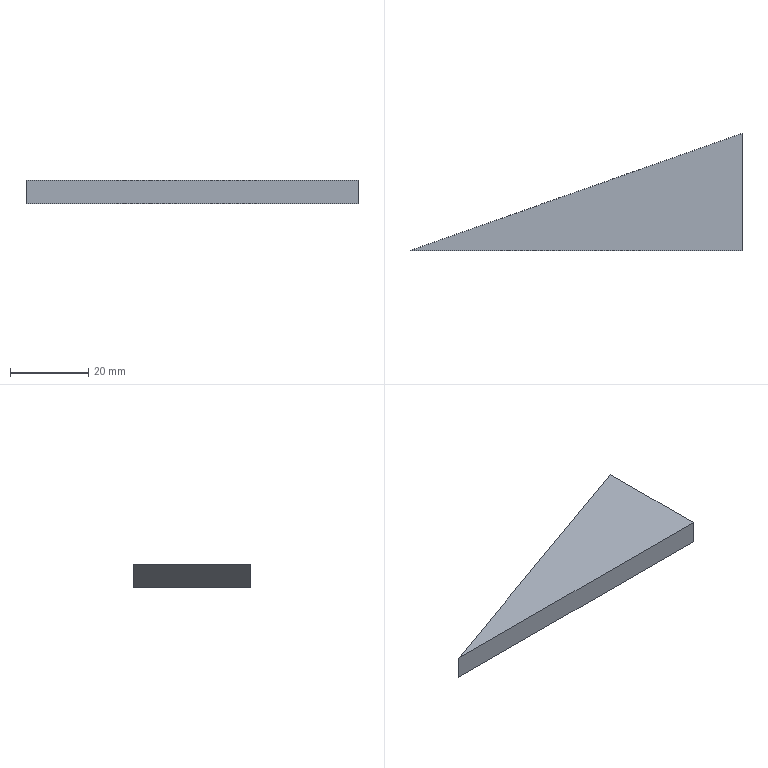Part | STEP file | Guide wheel mechanism revised.sldasm-Part-63 | 1 solid | 5 faces | box 85 x 30 x 6 mm | volume 7650 mm3 | plane 5
STEP:
#1=CARTESIAN_POINT('',(-42.5,7.,-40.5));
#2=VERTEX_POINT('',#1);
#3=CARTESIAN_POINT('',(42.5,37.,-40.5));
#4=VERTEX_POINT('',#3);
#5=CARTESIAN_POINT('',(-42.5,7.,-40.5));
#6=DIRECTION('',(0.943,0.3328,0.));
#7=VECTOR('',#6,1000.);
#8=LINE('',#5,#7);
#9=EDGE_CURVE('',#2,#4,#8,.T.);
#10=ORIENTED_EDGE('',*,*,#9,.F.);
#11=CARTESIAN_POINT('',(-42.5,7.,-34.5));
#12=VERTEX_POINT('',#11);
#13=CARTESIAN_POINT('',(-42.5,7.,-34.5));
#14=DIRECTION('',(0.,0.,-1.));
#15=VECTOR('',#14,1000.);
#16=LINE('',#13,#15);
#17=EDGE_CURVE('',#12,#2,#16,.T.);
#18=ORIENTED_EDGE('',*,*,#17,.F.);
#19=CARTESIAN_POINT('',(42.5,37.,-34.5));
#20=VERTEX_POINT('',#19);
#21=CARTESIAN_POINT('',(-42.5,7.,-34.5));
#22=DIRECTION('',(0.943,0.3328,0.));
#23=VECTOR('',#22,1000.);
#24=LINE('',#21,#23);
#25=EDGE_CURVE('',#12,#20,#24,.T.);
#26=ORIENTED_EDGE('',*,*,#25,.T.);
#27=CARTESIAN_POINT('',(42.5,37.,-34.5));
#28=DIRECTION('',(0.,0.,-1.));
#29=VECTOR('',#28,1000.);
#30=LINE('',#27,#29);
#31=EDGE_CURVE('',#20,#4,#30,.T.);
#32=ORIENTED_EDGE('',*,*,#31,.T.);
#33=EDGE_LOOP('',(#10,#18,#26,#32));
#34=FACE_OUTER_BOUND('',#33,.T.);
#35=CARTESIAN_POINT('',(-42.5,7.,-34.5));
#36=DIRECTION('',(-0.3328,0.943,0.));
#37=DIRECTION('',(-0.943,-0.3328,0.));
#38=AXIS2_PLACEMENT_3D('',#35,#36,#37);
#39=PLANE('',#38);
#40=ADVANCED_FACE('',(#34),#39,.T.);
#41=CARTESIAN_POINT('',(42.5,7.,-40.5));
#42=VERTEX_POINT('',#41);
#43=CARTESIAN_POINT('',(42.5,7.,-40.5));
#44=DIRECTION('',(-1.,0.,0.));
#45=VECTOR('',#44,1000.);
#46=LINE('',#43,#45);
#47=EDGE_CURVE('',#42,#2,#46,.T.);
#48=ORIENTED_EDGE('',*,*,#47,.F.);
#49=CARTESIAN_POINT('',(42.5,7.,-34.5));
#50=VERTEX_POINT('',#49);
#51=CARTESIAN_POINT('',(42.5,7.,-34.5));
#52=DIRECTION('',(0.,0.,-1.));
#53=VECTOR('',#52,1000.);
#54=LINE('',#51,#53);
#55=EDGE_CURVE('',#50,#42,#54,.T.);
#56=ORIENTED_EDGE('',*,*,#55,.F.);
#57=CARTESIAN_POINT('',(42.5,7.,-34.5));
#58=DIRECTION('',(-1.,0.,0.));
#59=VECTOR('',#58,1000.);
#60=LINE('',#57,#59);
#61=EDGE_CURVE('',#50,#12,#60,.T.);
#62=ORIENTED_EDGE('',*,*,#61,.T.);
#63=ORIENTED_EDGE('',*,*,#17,.T.);
#64=EDGE_LOOP('',(#48,#56,#62,#63));
#65=FACE_OUTER_BOUND('',#64,.T.);
#66=CARTESIAN_POINT('',(42.5,7.,-34.5));
#67=DIRECTION('',(0.,-1.,0.));
#68=DIRECTION('',(0.,0.,-1.));
#69=AXIS2_PLACEMENT_3D('',#66,#67,#68);
#70=PLANE('',#69);
#71=ADVANCED_FACE('',(#65),#70,.T.);
#72=CARTESIAN_POINT('',(42.5,37.,-40.5));
#73=DIRECTION('',(0.,-1.,0.));
#74=VECTOR('',#73,1000.);
#75=LINE('',#72,#74);
#76=EDGE_CURVE('',#4,#42,#75,.T.);
#77=ORIENTED_EDGE('',*,*,#76,.F.);
#78=ORIENTED_EDGE('',*,*,#31,.F.);
#79=CARTESIAN_POINT('',(42.5,37.,-34.5));
#80=DIRECTION('',(0.,-1.,0.));
#81=VECTOR('',#80,1000.);
#82=LINE('',#79,#81);
#83=EDGE_CURVE('',#20,#50,#82,.T.);
#84=ORIENTED_EDGE('',*,*,#83,.T.);
#85=ORIENTED_EDGE('',*,*,#55,.T.);
#86=EDGE_LOOP('',(#77,#78,#84,#85));
#87=FACE_OUTER_BOUND('',#86,.T.);
#88=CARTESIAN_POINT('',(42.5,37.,-34.5));
#89=DIRECTION('',(1.,0.,0.));
#90=DIRECTION('',(0.,0.,-1.));
#91=AXIS2_PLACEMENT_3D('',#88,#89,#90);
#92=PLANE('',#91);
#93=ADVANCED_FACE('',(#87),#92,.T.);
#94=ORIENTED_EDGE('',*,*,#25,.F.);
#95=ORIENTED_EDGE('',*,*,#61,.F.);
#96=ORIENTED_EDGE('',*,*,#83,.F.);
#97=EDGE_LOOP('',(#94,#95,#96));
#98=FACE_OUTER_BOUND('',#97,.T.);
#99=CARTESIAN_POINT('',(0.,0.,-34.5));
#100=DIRECTION('',(0.,0.,-1.));
#101=DIRECTION('',(0.,1.,0.));
#102=AXIS2_PLACEMENT_3D('',#99,#100,#101);
#103=PLANE('',#102);
#104=ADVANCED_FACE('',(#98),#103,.F.);
#105=ORIENTED_EDGE('',*,*,#9,.T.);
#106=ORIENTED_EDGE('',*,*,#76,.T.);
#107=ORIENTED_EDGE('',*,*,#47,.T.);
#108=EDGE_LOOP('',(#105,#106,#107));
#109=FACE_OUTER_BOUND('',#108,.T.);
#110=CARTESIAN_POINT('',(0.,0.,-40.5));
#111=DIRECTION('',(0.,0.,-1.));
#112=DIRECTION('',(0.,1.,0.));
#113=AXIS2_PLACEMENT_3D('',#110,#111,#112);
#114=PLANE('',#113);
#115=ADVANCED_FACE('',(#109),#114,.T.);
#116=CLOSED_SHELL('',(#40,#71,#93,#104,#115));
#117=MANIFOLD_SOLID_BREP('',#116);
#118=CARTESIAN_POINT('',(0.,0.,0.));
#119=DIRECTION('',(0.,0.,1.));
#120=DIRECTION('',(1.,0.,0.));
#121=AXIS2_PLACEMENT_3D('',#118,#119,#120);
#122=(LENGTH_UNIT()NAMED_UNIT(*)SI_UNIT(.MILLI.,.METRE.));
#123=UNCERTAINTY_MEASURE_WITH_UNIT(LENGTH_MEASURE(0.00001),#122,'','');
#124=(NAMED_UNIT(*)PLANE_ANGLE_UNIT()SI_UNIT($,.RADIAN.));
#125=(NAMED_UNIT(*)SI_UNIT($,.STERADIAN.)SOLID_ANGLE_UNIT());
#126=(GEOMETRIC_REPRESENTATION_CONTEXT(3)GLOBAL_UNCERTAINTY_ASSIGNED_CONTEXT((#123))GLOBAL_UNIT_ASSIGNED_CONTEXT((#122,#124,#125))REPRESENTATION_CONTEXT('',''));
#127=ADVANCED_BREP_SHAPE_REPRESENTATION('',(#117,#121),#126);